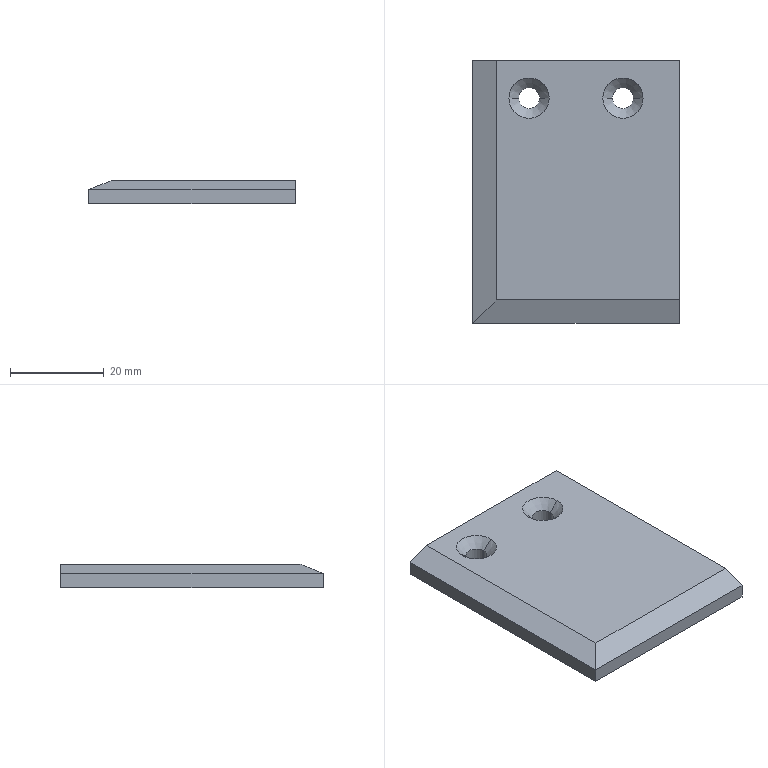Part | STEP file | PN_0027 Mount electronic clip acrylic plate | 1 solid | 16 faces | box 44 x 56 x 5 mm | volume 11600 mm3 | plane 8 | cone 4 | cylinder 4 | commonest cylinder face diameters 4.5 x4
STEP:
#1=CARTESIAN_POINT('',(0.,0.,0.));
#2=DIRECTION('',(0.,0.,1.));
#3=DIRECTION('',(1.,0.,0.));
#4=AXIS2_PLACEMENT_3D('',#1,#2,#3);
#5=CARTESIAN_POINT('',(-7.75,20.,2.95));
#6=VERTEX_POINT('',#5);
#7=CARTESIAN_POINT('',(-5.7,20.,5.));
#8=VERTEX_POINT('',#7);
#9=CARTESIAN_POINT('',(-5.7,20.,5.));
#10=DIRECTION('',(0.7071,0.,0.7071));
#11=VECTOR('',#10,1.);
#12=LINE('',#9,#11);
#13=CARTESIAN_POINT('',(-10.,20.,5.));
#14=DIRECTION('',(0.,0.,1.));
#15=DIRECTION('',(1.,0.,0.));
#16=AXIS2_PLACEMENT_3D('',#13,#14,#15);
#17=CONICAL_SURFACE('',#16,4.3,0.7854);
#18=CARTESIAN_POINT('',(6.283,0.));
#19=DIRECTION('',(0.,1.));
#20=VECTOR('',#19,1.);
#21=LINE('',#18,#20);
#22=(GEOMETRIC_REPRESENTATION_CONTEXT(2)PARAMETRIC_REPRESENTATION_CONTEXT()REPRESENTATION_CONTEXT('',''));
#23=DEFINITIONAL_REPRESENTATION('',(#21),#22);
#24=PCURVE('',#17,#23);
#25=CARTESIAN_POINT('',(-10.,20.,5.));
#26=DIRECTION('',(0.,0.,1.));
#27=DIRECTION('',(1.,0.,0.));
#28=AXIS2_PLACEMENT_3D('',#25,#26,#27);
#29=CONICAL_SURFACE('',#28,4.3,0.7854);
#30=CARTESIAN_POINT('',(0.,0.));
#31=DIRECTION('',(0.,1.));
#32=VECTOR('',#31,1.);
#33=LINE('',#30,#32);
#34=(GEOMETRIC_REPRESENTATION_CONTEXT(2)PARAMETRIC_REPRESENTATION_CONTEXT()REPRESENTATION_CONTEXT('',''));
#35=DEFINITIONAL_REPRESENTATION('',(#33),#34);
#36=PCURVE('',#29,#35);
#37=SURFACE_CURVE('',#12,(#24,#36),.PCURVE_S1.);
#38=EDGE_CURVE('',#6,#8,#37,.T.);
#39=ORIENTED_EDGE('',*,*,#38,.T.);
#40=CARTESIAN_POINT('',(-14.3,20.,5.));
#41=VERTEX_POINT('',#40);
#42=CARTESIAN_POINT('',(-10.,20.,5.));
#43=DIRECTION('',(0.,0.,1.));
#44=DIRECTION('',(1.,0.,0.));
#45=AXIS2_PLACEMENT_3D('',#42,#43,#44);
#46=CIRCLE('',#45,4.3);
#47=CARTESIAN_POINT('',(0.,0.));
#48=DIRECTION('',(1.,0.));
#49=VECTOR('',#48,1.);
#50=LINE('',#47,#49);
#51=(GEOMETRIC_REPRESENTATION_CONTEXT(2)PARAMETRIC_REPRESENTATION_CONTEXT()REPRESENTATION_CONTEXT('',''));
#52=DEFINITIONAL_REPRESENTATION('',(#50),#51);
#53=PCURVE('',#17,#52);
#54=CARTESIAN_POINT('',(0.,0.,5.));
#55=DIRECTION('',(0.,0.,-1.));
#56=DIRECTION('',(-1.,0.,0.));
#57=AXIS2_PLACEMENT_3D('',#54,#55,#56);
#58=PLANE('',#57);
#59=CARTESIAN_POINT('',(5.7,20.));
#60=CARTESIAN_POINT('',(5.7,27.448));
#61=CARTESIAN_POINT('',(12.15,23.724));
#62=CARTESIAN_POINT('',(18.6,20.));
#63=CARTESIAN_POINT('',(12.15,16.276));
#64=CARTESIAN_POINT('',(5.7,12.552));
#65=CARTESIAN_POINT('',(5.7,20.));
#66=(BOUNDED_CURVE()B_SPLINE_CURVE(2,(#59,#60,#61,#62,#63,#64,#65),.UNSPECIFIED.,.T.,.F.)B_SPLINE_CURVE_WITH_KNOTS((1,2,2,2,2,1),(-2.094,0.,2.094,4.189,6.283,8.378),.UNSPECIFIED.)CURVE()GEOMETRIC_REPRESENTATION_ITEM()RATIONAL_B_SPLINE_CURVE((1.,0.5,1.,0.5,1.,0.5,1.))REPRESENTATION_ITEM(''));
#67=(GEOMETRIC_REPRESENTATION_CONTEXT(2)PARAMETRIC_REPRESENTATION_CONTEXT()REPRESENTATION_CONTEXT('',''));
#68=DEFINITIONAL_REPRESENTATION('',(#66),#67);
#69=PCURVE('',#58,#68);
#70=SURFACE_CURVE('',#46,(#53,#69),.PCURVE_S1.);
#71=EDGE_CURVE('',#41,#8,#70,.T.);
#72=ORIENTED_EDGE('',*,*,#71,.F.);
#73=CARTESIAN_POINT('',(-12.25,20.,2.95));
#74=VERTEX_POINT('',#73);
#75=CARTESIAN_POINT('',(-14.3,20.,5.));
#76=DIRECTION('',(-0.7071,0.,0.7071));
#77=VECTOR('',#76,1.);
#78=LINE('',#75,#77);
#79=CARTESIAN_POINT('',(3.142,0.));
#80=DIRECTION('',(0.,1.));
#81=VECTOR('',#80,1.);
#82=LINE('',#79,#81);
#83=(GEOMETRIC_REPRESENTATION_CONTEXT(2)PARAMETRIC_REPRESENTATION_CONTEXT()REPRESENTATION_CONTEXT('',''));
#84=DEFINITIONAL_REPRESENTATION('',(#82),#83);
#85=PCURVE('',#17,#84);
#86=CARTESIAN_POINT('',(3.142,0.));
#87=DIRECTION('',(0.,1.));
#88=VECTOR('',#87,1.);
#89=LINE('',#86,#88);
#90=(GEOMETRIC_REPRESENTATION_CONTEXT(2)PARAMETRIC_REPRESENTATION_CONTEXT()REPRESENTATION_CONTEXT('',''));
#91=DEFINITIONAL_REPRESENTATION('',(#89),#90);
#92=PCURVE('',#29,#91);
#93=SURFACE_CURVE('',#78,(#85,#92),.PCURVE_S1.);
#94=EDGE_CURVE('',#74,#41,#93,.T.);
#95=ORIENTED_EDGE('',*,*,#94,.F.);
#96=CARTESIAN_POINT('',(-10.,20.,2.95));
#97=DIRECTION('',(0.,0.,1.));
#98=DIRECTION('',(1.,0.,0.));
#99=AXIS2_PLACEMENT_3D('',#96,#97,#98);
#100=CIRCLE('',#99,2.25);
#101=CARTESIAN_POINT('',(0.,-2.05));
#102=DIRECTION('',(1.,0.));
#103=VECTOR('',#102,1.);
#104=LINE('',#101,#103);
#105=(GEOMETRIC_REPRESENTATION_CONTEXT(2)PARAMETRIC_REPRESENTATION_CONTEXT()REPRESENTATION_CONTEXT('',''));
#106=DEFINITIONAL_REPRESENTATION('',(#104),#105);
#107=PCURVE('',#17,#106);
#108=CARTESIAN_POINT('',(-10.,20.,5.));
#109=DIRECTION('',(0.,0.,1.));
#110=DIRECTION('',(1.,0.,0.));
#111=AXIS2_PLACEMENT_3D('',#108,#109,#110);
#112=CYLINDRICAL_SURFACE('',#111,2.25);
#113=CARTESIAN_POINT('',(0.,-2.05));
#114=DIRECTION('',(1.,0.));
#115=VECTOR('',#114,1.);
#116=LINE('',#113,#115);
#117=(GEOMETRIC_REPRESENTATION_CONTEXT(2)PARAMETRIC_REPRESENTATION_CONTEXT()REPRESENTATION_CONTEXT('',''));
#118=DEFINITIONAL_REPRESENTATION('',(#116),#117);
#119=PCURVE('',#112,#118);
#120=SURFACE_CURVE('',#100,(#107,#119),.PCURVE_S1.);
#121=EDGE_CURVE('',#74,#6,#120,.T.);
#122=ORIENTED_EDGE('',*,*,#121,.T.);
#123=EDGE_LOOP('',(#39,#72,#95,#122));
#124=FACE_BOUND('',#123,.F.);
#125=ADVANCED_FACE('',(#124),#17,.F.);
#126=CARTESIAN_POINT('',(-7.75,20.,0.));
#127=VERTEX_POINT('',#126);
#128=CARTESIAN_POINT('',(-7.75,20.,5.));
#129=DIRECTION('',(0.,0.,1.));
#130=VECTOR('',#129,1.);
#131=LINE('',#128,#130);
#132=CARTESIAN_POINT('',(6.283,0.));
#133=DIRECTION('',(0.,1.));
#134=VECTOR('',#133,1.);
#135=LINE('',#132,#134);
#136=(GEOMETRIC_REPRESENTATION_CONTEXT(2)PARAMETRIC_REPRESENTATION_CONTEXT()REPRESENTATION_CONTEXT('',''));
#137=DEFINITIONAL_REPRESENTATION('',(#135),#136);
#138=PCURVE('',#112,#137);
#139=CARTESIAN_POINT('',(-10.,20.,5.));
#140=DIRECTION('',(0.,0.,1.));
#141=DIRECTION('',(1.,0.,0.));
#142=AXIS2_PLACEMENT_3D('',#139,#140,#141);
#143=CYLINDRICAL_SURFACE('',#142,2.25);
#144=CARTESIAN_POINT('',(0.,0.));
#145=DIRECTION('',(0.,1.));
#146=VECTOR('',#145,1.);
#147=LINE('',#144,#146);
#148=(GEOMETRIC_REPRESENTATION_CONTEXT(2)PARAMETRIC_REPRESENTATION_CONTEXT()REPRESENTATION_CONTEXT('',''));
#149=DEFINITIONAL_REPRESENTATION('',(#147),#148);
#150=PCURVE('',#143,#149);
#151=SURFACE_CURVE('',#131,(#138,#150),.PCURVE_S1.);
#152=EDGE_CURVE('',#127,#6,#151,.T.);
#153=ORIENTED_EDGE('',*,*,#152,.T.);
#154=ORIENTED_EDGE('',*,*,#121,.F.);
#155=CARTESIAN_POINT('',(-12.25,20.,0.));
#156=VERTEX_POINT('',#155);
#157=CARTESIAN_POINT('',(-12.25,20.,5.));
#158=DIRECTION('',(0.,0.,1.));
#159=VECTOR('',#158,1.);
#160=LINE('',#157,#159);
#161=CARTESIAN_POINT('',(3.142,0.));
#162=DIRECTION('',(0.,1.));
#163=VECTOR('',#162,1.);
#164=LINE('',#161,#163);
#165=(GEOMETRIC_REPRESENTATION_CONTEXT(2)PARAMETRIC_REPRESENTATION_CONTEXT()REPRESENTATION_CONTEXT('',''));
#166=DEFINITIONAL_REPRESENTATION('',(#164),#165);
#167=PCURVE('',#112,#166);
#168=CARTESIAN_POINT('',(3.142,0.));
#169=DIRECTION('',(0.,1.));
#170=VECTOR('',#169,1.);
#171=LINE('',#168,#170);
#172=(GEOMETRIC_REPRESENTATION_CONTEXT(2)PARAMETRIC_REPRESENTATION_CONTEXT()REPRESENTATION_CONTEXT('',''));
#173=DEFINITIONAL_REPRESENTATION('',(#171),#172);
#174=PCURVE('',#143,#173);
#175=SURFACE_CURVE('',#160,(#167,#174),.PCURVE_S1.);
#176=EDGE_CURVE('',#156,#74,#175,.T.);
#177=ORIENTED_EDGE('',*,*,#176,.F.);
#178=CARTESIAN_POINT('',(-10.,20.,0.));
#179=DIRECTION('',(0.,0.,1.));
#180=DIRECTION('',(1.,0.,0.));
#181=AXIS2_PLACEMENT_3D('',#178,#179,#180);
#182=CIRCLE('',#181,2.25);
#183=CARTESIAN_POINT('',(0.,-5.));
#184=DIRECTION('',(1.,0.));
#185=VECTOR('',#184,1.);
#186=LINE('',#183,#185);
#187=(GEOMETRIC_REPRESENTATION_CONTEXT(2)PARAMETRIC_REPRESENTATION_CONTEXT()REPRESENTATION_CONTEXT('',''));
#188=DEFINITIONAL_REPRESENTATION('',(#186),#187);
#189=PCURVE('',#112,#188);
#190=CARTESIAN_POINT('',(0.,0.,0.));
#191=DIRECTION('',(0.,0.,-1.));
#192=DIRECTION('',(-1.,0.,0.));
#193=AXIS2_PLACEMENT_3D('',#190,#191,#192);
#194=PLANE('',#193);
#195=CARTESIAN_POINT('',(7.75,20.));
#196=CARTESIAN_POINT('',(7.75,23.897));
#197=CARTESIAN_POINT('',(11.125,21.949));
#198=CARTESIAN_POINT('',(14.5,20.));
#199=CARTESIAN_POINT('',(11.125,18.051));
#200=CARTESIAN_POINT('',(7.75,16.103));
#201=CARTESIAN_POINT('',(7.75,20.));
#202=(BOUNDED_CURVE()B_SPLINE_CURVE(2,(#195,#196,#197,#198,#199,#200,#201),.UNSPECIFIED.,.T.,.F.)B_SPLINE_CURVE_WITH_KNOTS((1,2,2,2,2,1),(-2.094,0.,2.094,4.189,6.283,8.378),.UNSPECIFIED.)CURVE()GEOMETRIC_REPRESENTATION_ITEM()RATIONAL_B_SPLINE_CURVE((1.,0.5,1.,0.5,1.,0.5,1.))REPRESENTATION_ITEM(''));
#203=(GEOMETRIC_REPRESENTATION_CONTEXT(2)PARAMETRIC_REPRESENTATION_CONTEXT()REPRESENTATION_CONTEXT('',''));
#204=DEFINITIONAL_REPRESENTATION('',(#202),#203);
#205=PCURVE('',#194,#204);
#206=SURFACE_CURVE('',#182,(#189,#205),.PCURVE_S1.);
#207=EDGE_CURVE('',#156,#127,#206,.T.);
#208=ORIENTED_EDGE('',*,*,#207,.T.);
#209=EDGE_LOOP('',(#153,#154,#177,#208));
#210=FACE_BOUND('',#209,.F.);
#211=ADVANCED_FACE('',(#210),#112,.F.);
#212=CARTESIAN_POINT('',(12.25,20.,2.95));
#213=VERTEX_POINT('',#212);
#214=CARTESIAN_POINT('',(14.3,20.,5.));
#215=VERTEX_POINT('',#214);
#216=CARTESIAN_POINT('',(14.3,20.,5.));
#217=DIRECTION('',(0.7071,0.,0.7071));
#218=VECTOR('',#217,1.);
#219=LINE('',#216,#218);
#220=CARTESIAN_POINT('',(10.,20.,5.));
#221=DIRECTION('',(0.,0.,1.));
#222=DIRECTION('',(1.,0.,0.));
#223=AXIS2_PLACEMENT_3D('',#220,#221,#222);
#224=CONICAL_SURFACE('',#223,4.3,0.7854);
#225=CARTESIAN_POINT('',(6.283,0.));
#226=DIRECTION('',(0.,1.));
#227=VECTOR('',#226,1.);
#228=LINE('',#225,#227);
#229=(GEOMETRIC_REPRESENTATION_CONTEXT(2)PARAMETRIC_REPRESENTATION_CONTEXT()REPRESENTATION_CONTEXT('',''));
#230=DEFINITIONAL_REPRESENTATION('',(#228),#229);
#231=PCURVE('',#224,#230);
#232=CARTESIAN_POINT('',(10.,20.,5.));
#233=DIRECTION('',(0.,0.,1.));
#234=DIRECTION('',(1.,0.,0.));
#235=AXIS2_PLACEMENT_3D('',#232,#233,#234);
#236=CONICAL_SURFACE('',#235,4.3,0.7854);
#237=CARTESIAN_POINT('',(0.,0.));
#238=DIRECTION('',(0.,1.));
#239=VECTOR('',#238,1.);
#240=LINE('',#237,#239);
#241=(GEOMETRIC_REPRESENTATION_CONTEXT(2)PARAMETRIC_REPRESENTATION_CONTEXT()REPRESENTATION_CONTEXT('',''));
#242=DEFINITIONAL_REPRESENTATION('',(#240),#241);
#243=PCURVE('',#236,#242);
#244=SURFACE_CURVE('',#219,(#231,#243),.PCURVE_S1.);
#245=EDGE_CURVE('',#213,#215,#244,.T.);
#246=ORIENTED_EDGE('',*,*,#245,.T.);
#247=CARTESIAN_POINT('',(5.7,20.,5.));
#248=VERTEX_POINT('',#247);
#249=CARTESIAN_POINT('',(10.,20.,5.));
#250=DIRECTION('',(0.,0.,1.));
#251=DIRECTION('',(1.,0.,0.));
#252=AXIS2_PLACEMENT_3D('',#249,#250,#251);
#253=CIRCLE('',#252,4.3);
#254=CARTESIAN_POINT('',(0.,0.));
#255=DIRECTION('',(1.,0.));
#256=VECTOR('',#255,1.);
#257=LINE('',#254,#256);
#258=(GEOMETRIC_REPRESENTATION_CONTEXT(2)PARAMETRIC_REPRESENTATION_CONTEXT()REPRESENTATION_CONTEXT('',''));
#259=DEFINITIONAL_REPRESENTATION('',(#257),#258);
#260=PCURVE('',#224,#259);
#261=CARTESIAN_POINT('',(-14.3,20.));
#262=CARTESIAN_POINT('',(-14.3,27.448));
#263=CARTESIAN_POINT('',(-7.85,23.724));
#264=CARTESIAN_POINT('',(-1.4,20.));
#265=CARTESIAN_POINT('',(-7.85,16.276));
#266=CARTESIAN_POINT('',(-14.3,12.552));
#267=CARTESIAN_POINT('',(-14.3,20.));
#268=(BOUNDED_CURVE()B_SPLINE_CURVE(2,(#261,#262,#263,#264,#265,#266,#267),.UNSPECIFIED.,.T.,.F.)B_SPLINE_CURVE_WITH_KNOTS((1,2,2,2,2,1),(-2.094,0.,2.094,4.189,6.283,8.378),.UNSPECIFIED.)CURVE()GEOMETRIC_REPRESENTATION_ITEM()RATIONAL_B_SPLINE_CURVE((1.,0.5,1.,0.5,1.,0.5,1.))REPRESENTATION_ITEM(''));
#269=(GEOMETRIC_REPRESENTATION_CONTEXT(2)PARAMETRIC_REPRESENTATION_CONTEXT()REPRESENTATION_CONTEXT('',''));
#270=DEFINITIONAL_REPRESENTATION('',(#268),#269);
#271=PCURVE('',#58,#270);
#272=SURFACE_CURVE('',#253,(#260,#271),.PCURVE_S1.);
#273=EDGE_CURVE('',#248,#215,#272,.T.);
#274=ORIENTED_EDGE('',*,*,#273,.F.);
#275=CARTESIAN_POINT('',(7.75,20.,2.95));
#276=VERTEX_POINT('',#275);
#277=CARTESIAN_POINT('',(5.7,20.,5.));
#278=DIRECTION('',(-0.7071,0.,0.7071));
#279=VECTOR('',#278,1.);
#280=LINE('',#277,#279);
#281=CARTESIAN_POINT('',(3.142,0.));
#282=DIRECTION('',(0.,1.));
#283=VECTOR('',#282,1.);
#284=LINE('',#281,#283);
#285=(GEOMETRIC_REPRESENTATION_CONTEXT(2)PARAMETRIC_REPRESENTATION_CONTEXT()REPRESENTATION_CONTEXT('',''));
#286=DEFINITIONAL_REPRESENTATION('',(#284),#285);
#287=PCURVE('',#224,#286);
#288=CARTESIAN_POINT('',(3.142,0.));
#289=DIRECTION('',(0.,1.));
#290=VECTOR('',#289,1.);
#291=LINE('',#288,#290);
#292=(GEOMETRIC_REPRESENTATION_CONTEXT(2)PARAMETRIC_REPRESENTATION_CONTEXT()REPRESENTATION_CONTEXT('',''));
#293=DEFINITIONAL_REPRESENTATION('',(#291),#292);
#294=PCURVE('',#236,#293);
#295=SURFACE_CURVE('',#280,(#287,#294),.PCURVE_S1.);
#296=EDGE_CURVE('',#276,#248,#295,.T.);
#297=ORIENTED_EDGE('',*,*,#296,.F.);
#298=CARTESIAN_POINT('',(10.,20.,2.95));
#299=DIRECTION('',(0.,0.,1.));
#300=DIRECTION('',(1.,0.,0.));
#301=AXIS2_PLACEMENT_3D('',#298,#299,#300);
#302=CIRCLE('',#301,2.25);
#303=CARTESIAN_POINT('',(0.,-2.05));
#304=DIRECTION('',(1.,0.));
#305=VECTOR('',#304,1.);
#306=LINE('',#303,#305);
#307=(GEOMETRIC_REPRESENTATION_CONTEXT(2)PARAMETRIC_REPRESENTATION_CONTEXT()REPRESENTATION_CONTEXT('',''));
#308=DEFINITIONAL_REPRESENTATION('',(#306),#307);
#309=PCURVE('',#224,#308);
#310=CARTESIAN_POINT('',(10.,20.,5.));
#311=DIRECTION('',(0.,0.,1.));
#312=DIRECTION('',(1.,0.,0.));
#313=AXIS2_PLACEMENT_3D('',#310,#311,#312);
#314=CYLINDRICAL_SURFACE('',#313,2.25);
#315=CARTESIAN_POINT('',(0.,-2.05));
#316=DIRECTION('',(1.,0.));
#317=VECTOR('',#316,1.);
#318=LINE('',#315,#317);
#319=(GEOMETRIC_REPRESENTATION_CONTEXT(2)PARAMETRIC_REPRESENTATION_CONTEXT()REPRESENTATION_CONTEXT('',''));
#320=DEFINITIONAL_REPRESENTATION('',(#318),#319);
#321=PCURVE('',#314,#320);
#322=SURFACE_CURVE('',#302,(#309,#321),.PCURVE_S1.);
#323=EDGE_CURVE('',#276,#213,#322,.T.);
#324=ORIENTED_EDGE('',*,*,#323,.T.);
#325=EDGE_LOOP('',(#246,#274,#297,#324));
#326=FACE_BOUND('',#325,.F.);
#327=ADVANCED_FACE('',(#326),#224,.F.);
#328=CARTESIAN_POINT('',(12.25,20.,0.));
#329=VERTEX_POINT('',#328);
#330=CARTESIAN_POINT('',(12.25,20.,5.));
#331=DIRECTION('',(0.,0.,1.));
#332=VECTOR('',#331,1.);
#333=LINE('',#330,#332);
#334=CARTESIAN_POINT('',(6.283,0.));
#335=DIRECTION('',(0.,1.));
#336=VECTOR('',#335,1.);
#337=LINE('',#334,#336);
#338=(GEOMETRIC_REPRESENTATION_CONTEXT(2)PARAMETRIC_REPRESENTATION_CONTEXT()REPRESENTATION_CONTEXT('',''));
#339=DEFINITIONAL_REPRESENTATION('',(#337),#338);
#340=PCURVE('',#314,#339);
#341=CARTESIAN_POINT('',(10.,20.,5.));
#342=DIRECTION('',(0.,0.,1.));
#343=DIRECTION('',(1.,0.,0.));
#344=AXIS2_PLACEMENT_3D('',#341,#342,#343);
#345=CYLINDRICAL_SURFACE('',#344,2.25);
#346=CARTESIAN_POINT('',(0.,0.));
#347=DIRECTION('',(0.,1.));
#348=VECTOR('',#347,1.);
#349=LINE('',#346,#348);
#350=(GEOMETRIC_REPRESENTATION_CONTEXT(2)PARAMETRIC_REPRESENTATION_CONTEXT()REPRESENTATION_CONTEXT('',''));
#351=DEFINITIONAL_REPRESENTATION('',(#349),#350);
#352=PCURVE('',#345,#351);
#353=SURFACE_CURVE('',#333,(#340,#352),.PCURVE_S1.);
#354=EDGE_CURVE('',#329,#213,#353,.T.);
#355=ORIENTED_EDGE('',*,*,#354,.T.);
#356=ORIENTED_EDGE('',*,*,#323,.F.);
#357=CARTESIAN_POINT('',(7.75,20.,0.));
#358=VERTEX_POINT('',#357);
#359=CARTESIAN_POINT('',(7.75,20.,5.));
#360=DIRECTION('',(0.,0.,1.));
#361=VECTOR('',#360,1.);
#362=LINE('',#359,#361);
#363=CARTESIAN_POINT('',(3.142,0.));
#364=DIRECTION('',(0.,1.));
#365=VECTOR('',#364,1.);
#366=LINE('',#363,#365);
#367=(GEOMETRIC_REPRESENTATION_CONTEXT(2)PARAMETRIC_REPRESENTATION_CONTEXT()REPRESENTATION_CONTEXT('',''));
#368=DEFINITIONAL_REPRESENTATION('',(#366),#367);
#369=PCURVE('',#314,#368);
#370=CARTESIAN_POINT('',(3.142,0.));
#371=DIRECTION('',(0.,1.));
#372=VECTOR('',#371,1.);
#373=LINE('',#370,#372);
#374=(GEOMETRIC_REPRESENTATION_CONTEXT(2)PARAMETRIC_REPRESENTATION_CONTEXT()REPRESENTATION_CONTEXT('',''));
#375=DEFINITIONAL_REPRESENTATION('',(#373),#374);
#376=PCURVE('',#345,#375);
#377=SURFACE_CURVE('',#362,(#369,#376),.PCURVE_S1.);
#378=EDGE_CURVE('',#358,#276,#377,.T.);
#379=ORIENTED_EDGE('',*,*,#378,.F.);
#380=CARTESIAN_POINT('',(10.,20.,0.));
#381=DIRECTION('',(0.,0.,1.));
#382=DIRECTION('',(1.,0.,0.));
#383=AXIS2_PLACEMENT_3D('',#380,#381,#382);
#384=CIRCLE('',#383,2.25);
#385=CARTESIAN_POINT('',(0.,-5.));
#386=DIRECTION('',(1.,0.));
#387=VECTOR('',#386,1.);
#388=LINE('',#385,#387);
#389=(GEOMETRIC_REPRESENTATION_CONTEXT(2)PARAMETRIC_REPRESENTATION_CONTEXT()REPRESENTATION_CONTEXT('',''));
#390=DEFINITIONAL_REPRESENTATION('',(#388),#389);
#391=PCURVE('',#314,#390);
#392=CARTESIAN_POINT('',(-12.25,20.));
#393=CARTESIAN_POINT('',(-12.25,23.897));
#394=CARTESIAN_POINT('',(-8.875,21.949));
#395=CARTESIAN_POINT('',(-5.5,20.));
#396=CARTESIAN_POINT('',(-8.875,18.051));
#397=CARTESIAN_POINT('',(-12.25,16.103));
#398=CARTESIAN_POINT('',(-12.25,20.));
#399=(BOUNDED_CURVE()B_SPLINE_CURVE(2,(#392,#393,#394,#395,#396,#397,#398),.UNSPECIFIED.,.T.,.F.)B_SPLINE_CURVE_WITH_KNOTS((1,2,2,2,2,1),(-2.094,0.,2.094,4.189,6.283,8.378),.UNSPECIFIED.)CURVE()GEOMETRIC_REPRESENTATION_ITEM()RATIONAL_B_SPLINE_CURVE((1.,0.5,1.,0.5,1.,0.5,1.))REPRESENTATION_ITEM(''));
#400=(GEOMETRIC_REPRESENTATION_CONTEXT(2)PARAMETRIC_REPRESENTATION_CONTEXT()REPRESENTATION_CONTEXT('',''));
#401=DEFINITIONAL_REPRESENTATION('',(#399),#400);
#402=PCURVE('',#194,#401);
#403=SURFACE_CURVE('',#384,(#391,#402),.PCURVE_S1.);
#404=EDGE_CURVE('',#358,#329,#403,.T.);
#405=ORIENTED_EDGE('',*,*,#404,.T.);
#406=EDGE_LOOP('',(#355,#356,#379,#405));
#407=FACE_BOUND('',#406,.F.);
#408=ADVANCED_FACE('',(#407),#314,.F.);
#409=CARTESIAN_POINT('',(22.,-23.,5.));
#410=VERTEX_POINT('',#409);
#411=CARTESIAN_POINT('',(22.,28.,5.));
#412=VERTEX_POINT('',#411);
#413=CARTESIAN_POINT('',(22.,-28.,5.));
#414=DIRECTION('',(0.,1.,0.));
#415=VECTOR('',#414,1.);
#416=LINE('',#413,#415);
#417=CARTESIAN_POINT('',(22.,-28.,5.));
#418=DIRECTION('',(-1.,0.,0.));
#419=DIRECTION('',(0.,0.,1.));
#420=AXIS2_PLACEMENT_3D('',#417,#418,#419);
#421=PLANE('',#420);
#422=CARTESIAN_POINT('',(0.,0.));
#423=DIRECTION('',(0.,1.));
#424=VECTOR('',#423,1.);
#425=LINE('',#422,#424);
#426=(GEOMETRIC_REPRESENTATION_CONTEXT(2)PARAMETRIC_REPRESENTATION_CONTEXT()REPRESENTATION_CONTEXT('',''));
#427=DEFINITIONAL_REPRESENTATION('',(#425),#426);
#428=PCURVE('',#421,#427);
#429=CARTESIAN_POINT('',(-22.,-28.));
#430=DIRECTION('',(0.,1.));
#431=VECTOR('',#430,1.);
#432=LINE('',#429,#431);
#433=(GEOMETRIC_REPRESENTATION_CONTEXT(2)PARAMETRIC_REPRESENTATION_CONTEXT()REPRESENTATION_CONTEXT('',''));
#434=DEFINITIONAL_REPRESENTATION('',(#432),#433);
#435=PCURVE('',#58,#434);
#436=SURFACE_CURVE('',#416,(#428,#435),.PCURVE_S1.);
#437=EDGE_CURVE('',#410,#412,#436,.T.);
#438=ORIENTED_EDGE('',*,*,#437,.F.);
#439=CARTESIAN_POINT('',(22.,-28.,3.));
#440=VERTEX_POINT('',#439);
#441=CARTESIAN_POINT('',(22.,-23.,5.));
#442=DIRECTION('',(0.,-0.9285,-0.3714));
#443=VECTOR('',#442,1.);
#444=LINE('',#441,#443);
#445=CARTESIAN_POINT('',(0.,5.));
#446=DIRECTION('',(-0.3714,-0.9285));
#447=VECTOR('',#446,1.);
#448=LINE('',#445,#447);
#449=(GEOMETRIC_REPRESENTATION_CONTEXT(2)PARAMETRIC_REPRESENTATION_CONTEXT()REPRESENTATION_CONTEXT('',''));
#450=DEFINITIONAL_REPRESENTATION('',(#448),#449);
#451=PCURVE('',#421,#450);
#452=CARTESIAN_POINT('',(0.,-23.,5.));
#453=DIRECTION('',(0.,0.3714,-0.9285));
#454=DIRECTION('',(1.,0.,0.));
#455=AXIS2_PLACEMENT_3D('',#452,#453,#454);
#456=PLANE('',#455);
#457=CARTESIAN_POINT('',(22.,0.));
#458=DIRECTION('',(0.,1.));
#459=VECTOR('',#458,1.);
#460=LINE('',#457,#459);
#461=(GEOMETRIC_REPRESENTATION_CONTEXT(2)PARAMETRIC_REPRESENTATION_CONTEXT()REPRESENTATION_CONTEXT('',''));
#462=DEFINITIONAL_REPRESENTATION('',(#460),#461);
#463=PCURVE('',#456,#462);
#464=SURFACE_CURVE('',#444,(#451,#463),.PCURVE_S1.);
#465=EDGE_CURVE('',#410,#440,#464,.T.);
#466=ORIENTED_EDGE('',*,*,#465,.T.);
#467=CARTESIAN_POINT('',(22.,-28.,0.));
#468=VERTEX_POINT('',#467);
#469=CARTESIAN_POINT('',(22.,-28.,5.));
#470=DIRECTION('',(0.,0.,-1.));
#471=VECTOR('',#470,1.);
#472=LINE('',#469,#471);
#473=CARTESIAN_POINT('',(0.,0.));
#474=DIRECTION('',(-1.,0.));
#475=VECTOR('',#474,1.);
#476=LINE('',#473,#475);
#477=(GEOMETRIC_REPRESENTATION_CONTEXT(2)PARAMETRIC_REPRESENTATION_CONTEXT()REPRESENTATION_CONTEXT('',''));
#478=DEFINITIONAL_REPRESENTATION('',(#476),#477);
#479=PCURVE('',#421,#478);
#480=CARTESIAN_POINT('',(-22.,-28.,5.));
#481=DIRECTION('',(0.,1.,0.));
#482=DIRECTION('',(0.,0.,1.));
#483=AXIS2_PLACEMENT_3D('',#480,#481,#482);
#484=PLANE('',#483);
#485=CARTESIAN_POINT('',(0.,44.));
#486=DIRECTION('',(-1.,0.));
#487=VECTOR('',#486,1.);
#488=LINE('',#485,#487);
#489=(GEOMETRIC_REPRESENTATION_CONTEXT(2)PARAMETRIC_REPRESENTATION_CONTEXT()REPRESENTATION_CONTEXT('',''));
#490=DEFINITIONAL_REPRESENTATION('',(#488),#489);
#491=PCURVE('',#484,#490);
#492=SURFACE_CURVE('',#472,(#479,#491),.PCURVE_S1.);
#493=EDGE_CURVE('',#440,#468,#492,.T.);
#494=ORIENTED_EDGE('',*,*,#493,.T.);
#495=CARTESIAN_POINT('',(22.,28.,0.));
#496=VERTEX_POINT('',#495);
#497=CARTESIAN_POINT('',(22.,-28.,0.));
#498=DIRECTION('',(0.,1.,0.));
#499=VECTOR('',#498,1.);
#500=LINE('',#497,#499);
#501=CARTESIAN_POINT('',(-5.,0.));
#502=DIRECTION('',(0.,1.));
#503=VECTOR('',#502,1.);
#504=LINE('',#501,#503);
#505=(GEOMETRIC_REPRESENTATION_CONTEXT(2)PARAMETRIC_REPRESENTATION_CONTEXT()REPRESENTATION_CONTEXT('',''));
#506=DEFINITIONAL_REPRESENTATION('',(#504),#505);
#507=PCURVE('',#421,#506);
#508=CARTESIAN_POINT('',(-22.,-28.));
#509=DIRECTION('',(0.,1.));
#510=VECTOR('',#509,1.);
#511=LINE('',#508,#510);
#512=(GEOMETRIC_REPRESENTATION_CONTEXT(2)PARAMETRIC_REPRESENTATION_CONTEXT()REPRESENTATION_CONTEXT('',''));
#513=DEFINITIONAL_REPRESENTATION('',(#511),#512);
#514=PCURVE('',#194,#513);
#515=SURFACE_CURVE('',#500,(#507,#514),.PCURVE_S1.);
#516=EDGE_CURVE('',#468,#496,#515,.T.);
#517=ORIENTED_EDGE('',*,*,#516,.T.);
#518=CARTESIAN_POINT('',(22.,28.,5.));
#519=DIRECTION('',(0.,0.,-1.));
#520=VECTOR('',#519,1.);
#521=LINE('',#518,#520);
#522=CARTESIAN_POINT('',(0.,56.));
#523=DIRECTION('',(-1.,0.));
#524=VECTOR('',#523,1.);
#525=LINE('',#522,#524);
#526=(GEOMETRIC_REPRESENTATION_CONTEXT(2)PARAMETRIC_REPRESENTATION_CONTEXT()REPRESENTATION_CONTEXT('',''));
#527=DEFINITIONAL_REPRESENTATION('',(#525),#526);
#528=PCURVE('',#421,#527);
#529=CARTESIAN_POINT('',(-22.,28.,5.));
#530=DIRECTION('',(0.,-1.,0.));
#531=DIRECTION('',(0.,0.,-1.));
#532=AXIS2_PLACEMENT_3D('',#529,#530,#531);
#533=PLANE('',#532);
#534=CARTESIAN_POINT('',(0.,44.));
#535=DIRECTION('',(1.,0.));
#536=VECTOR('',#535,1.);
#537=LINE('',#534,#536);
#538=(GEOMETRIC_REPRESENTATION_CONTEXT(2)PARAMETRIC_REPRESENTATION_CONTEXT()REPRESENTATION_CONTEXT('',''));
#539=DEFINITIONAL_REPRESENTATION('',(#537),#538);
#540=PCURVE('',#533,#539);
#541=SURFACE_CURVE('',#521,(#528,#540),.PCURVE_S1.);
#542=EDGE_CURVE('',#412,#496,#541,.T.);
#543=ORIENTED_EDGE('',*,*,#542,.F.);
#544=EDGE_LOOP('',(#438,#466,#494,#517,#543));
#545=FACE_BOUND('',#544,.T.);
#546=ADVANCED_FACE('',(#545),#421,.F.);
#547=CARTESIAN_POINT('',(-22.,28.,3.));
#548=VERTEX_POINT('',#547);
#549=CARTESIAN_POINT('',(-22.,28.,0.));
#550=VERTEX_POINT('',#549);
#551=CARTESIAN_POINT('',(-22.,28.,5.));
#552=DIRECTION('',(0.,0.,-1.));
#553=VECTOR('',#552,1.);
#554=LINE('',#551,#553);
#555=CARTESIAN_POINT('',(0.,0.));
#556=DIRECTION('',(1.,0.));
#557=VECTOR('',#556,1.);
#558=LINE('',#555,#557);
#559=(GEOMETRIC_REPRESENTATION_CONTEXT(2)PARAMETRIC_REPRESENTATION_CONTEXT()REPRESENTATION_CONTEXT('',''));
#560=DEFINITIONAL_REPRESENTATION('',(#558),#559);
#561=PCURVE('',#533,#560);
#562=CARTESIAN_POINT('',(-22.,-28.,5.));
#563=DIRECTION('',(1.,0.,0.));
#564=DIRECTION('',(0.,0.,-1.));
#565=AXIS2_PLACEMENT_3D('',#562,#563,#564);
#566=PLANE('',#565);
#567=CARTESIAN_POINT('',(0.,56.));
#568=DIRECTION('',(1.,0.));
#569=VECTOR('',#568,1.);
#570=LINE('',#567,#569);
#571=(GEOMETRIC_REPRESENTATION_CONTEXT(2)PARAMETRIC_REPRESENTATION_CONTEXT()REPRESENTATION_CONTEXT('',''));
#572=DEFINITIONAL_REPRESENTATION('',(#570),#571);
#573=PCURVE('',#566,#572);
#574=SURFACE_CURVE('',#554,(#561,#573),.PCURVE_S1.);
#575=EDGE_CURVE('',#548,#550,#574,.T.);
#576=ORIENTED_EDGE('',*,*,#575,.F.);
#577=CARTESIAN_POINT('',(-17.,28.,5.));
#578=VERTEX_POINT('',#577);
#579=CARTESIAN_POINT('',(-17.,28.,5.));
#580=DIRECTION('',(0.9285,0.,0.3714));
#581=VECTOR('',#580,1.);
#582=LINE('',#579,#581);
#583=CARTESIAN_POINT('',(0.,5.));
#584=DIRECTION('',(-0.3714,0.9285));
#585=VECTOR('',#584,1.);
#586=LINE('',#583,#585);
#587=(GEOMETRIC_REPRESENTATION_CONTEXT(2)PARAMETRIC_REPRESENTATION_CONTEXT()REPRESENTATION_CONTEXT('',''));
#588=DEFINITIONAL_REPRESENTATION('',(#586),#587);
#589=PCURVE('',#533,#588);
#590=CARTESIAN_POINT('',(-17.,0.,5.));
#591=DIRECTION('',(0.3714,0.,-0.9285));
#592=DIRECTION('',(0.,-1.,0.));
#593=AXIS2_PLACEMENT_3D('',#590,#591,#592);
#594=PLANE('',#593);
#595=CARTESIAN_POINT('',(-28.,0.));
#596=DIRECTION('',(0.,-1.));
#597=VECTOR('',#596,1.);
#598=LINE('',#595,#597);
#599=(GEOMETRIC_REPRESENTATION_CONTEXT(2)PARAMETRIC_REPRESENTATION_CONTEXT()REPRESENTATION_CONTEXT('',''));
#600=DEFINITIONAL_REPRESENTATION('',(#598),#599);
#601=PCURVE('',#594,#600);
#602=SURFACE_CURVE('',#582,(#589,#601),.PCURVE_S1.);
#603=EDGE_CURVE('',#548,#578,#602,.T.);
#604=ORIENTED_EDGE('',*,*,#603,.T.);
#605=CARTESIAN_POINT('',(-22.,28.,5.));
#606=DIRECTION('',(-1.,0.,0.));
#607=VECTOR('',#606,1.);
#608=LINE('',#605,#607);
#609=CARTESIAN_POINT('',(0.,0.));
#610=DIRECTION('',(0.,-1.));
#611=VECTOR('',#610,1.);
#612=LINE('',#609,#611);
#613=(GEOMETRIC_REPRESENTATION_CONTEXT(2)PARAMETRIC_REPRESENTATION_CONTEXT()REPRESENTATION_CONTEXT('',''));
#614=DEFINITIONAL_REPRESENTATION('',(#612),#613);
#615=PCURVE('',#533,#614);
#616=CARTESIAN_POINT('',(22.,28.));
#617=DIRECTION('',(1.,0.));
#618=VECTOR('',#617,1.);
#619=LINE('',#616,#618);
#620=(GEOMETRIC_REPRESENTATION_CONTEXT(2)PARAMETRIC_REPRESENTATION_CONTEXT()REPRESENTATION_CONTEXT('',''));
#621=DEFINITIONAL_REPRESENTATION('',(#619),#620);
#622=PCURVE('',#58,#621);
#623=SURFACE_CURVE('',#608,(#615,#622),.PCURVE_S1.);
#624=EDGE_CURVE('',#412,#578,#623,.T.);
#625=ORIENTED_EDGE('',*,*,#624,.F.);
#626=ORIENTED_EDGE('',*,*,#542,.T.);
#627=CARTESIAN_POINT('',(-22.,28.,0.));
#628=DIRECTION('',(-1.,0.,0.));
#629=VECTOR('',#628,1.);
#630=LINE('',#627,#629);
#631=CARTESIAN_POINT('',(5.,0.));
#632=DIRECTION('',(0.,-1.));
#633=VECTOR('',#632,1.);
#634=LINE('',#631,#633);
#635=(GEOMETRIC_REPRESENTATION_CONTEXT(2)PARAMETRIC_REPRESENTATION_CONTEXT()REPRESENTATION_CONTEXT('',''));
#636=DEFINITIONAL_REPRESENTATION('',(#634),#635);
#637=PCURVE('',#533,#636);
#638=CARTESIAN_POINT('',(22.,28.));
#639=DIRECTION('',(1.,0.));
#640=VECTOR('',#639,1.);
#641=LINE('',#638,#640);
#642=(GEOMETRIC_REPRESENTATION_CONTEXT(2)PARAMETRIC_REPRESENTATION_CONTEXT()REPRESENTATION_CONTEXT('',''));
#643=DEFINITIONAL_REPRESENTATION('',(#641),#642);
#644=PCURVE('',#194,#643);
#645=SURFACE_CURVE('',#630,(#637,#644),.PCURVE_S1.);
#646=EDGE_CURVE('',#496,#550,#645,.T.);
#647=ORIENTED_EDGE('',*,*,#646,.T.);
#648=EDGE_LOOP('',(#576,#604,#625,#626,#647));
#649=FACE_BOUND('',#648,.T.);
#650=ADVANCED_FACE('',(#649),#533,.F.);
#651=CARTESIAN_POINT('',(-22.,-28.,3.));
#652=VERTEX_POINT('',#651);
#653=CARTESIAN_POINT('',(-22.,-28.,0.));
#654=VERTEX_POINT('',#653);
#655=CARTESIAN_POINT('',(-22.,-28.,5.));
#656=DIRECTION('',(0.,0.,-1.));
#657=VECTOR('',#656,1.);
#658=LINE('',#655,#657);
#659=CARTESIAN_POINT('',(0.,0.));
#660=DIRECTION('',(1.,0.));
#661=VECTOR('',#660,1.);
#662=LINE('',#659,#661);
#663=(GEOMETRIC_REPRESENTATION_CONTEXT(2)PARAMETRIC_REPRESENTATION_CONTEXT()REPRESENTATION_CONTEXT('',''));
#664=DEFINITIONAL_REPRESENTATION('',(#662),#663);
#665=PCURVE('',#566,#664);
#666=CARTESIAN_POINT('',(0.,0.));
#667=DIRECTION('',(-1.,0.));
#668=VECTOR('',#667,1.);
#669=LINE('',#666,#668);
#670=(GEOMETRIC_REPRESENTATION_CONTEXT(2)PARAMETRIC_REPRESENTATION_CONTEXT()REPRESENTATION_CONTEXT('',''));
#671=DEFINITIONAL_REPRESENTATION('',(#669),#670);
#672=PCURVE('',#484,#671);
#673=SURFACE_CURVE('',#658,(#665,#672),.PCURVE_S1.);
#674=EDGE_CURVE('',#652,#654,#673,.T.);
#675=ORIENTED_EDGE('',*,*,#674,.F.);
#676=CARTESIAN_POINT('',(-22.,-28.,3.));
#677=DIRECTION('',(0.,1.,0.));
#678=VECTOR('',#677,1.);
#679=LINE('',#676,#678);
#680=CARTESIAN_POINT('',(2.,0.));
#681=DIRECTION('',(0.,1.));
#682=VECTOR('',#681,1.);
#683=LINE('',#680,#682);
#684=(GEOMETRIC_REPRESENTATION_CONTEXT(2)PARAMETRIC_REPRESENTATION_CONTEXT()REPRESENTATION_CONTEXT('',''));
#685=DEFINITIONAL_REPRESENTATION('',(#683),#684);
#686=PCURVE('',#566,#685);
#687=CARTESIAN_POINT('',(28.,5.385));
#688=DIRECTION('',(-1.,0.));
#689=VECTOR('',#688,1.);
#690=LINE('',#687,#689);
#691=(GEOMETRIC_REPRESENTATION_CONTEXT(2)PARAMETRIC_REPRESENTATION_CONTEXT()REPRESENTATION_CONTEXT('',''));
#692=DEFINITIONAL_REPRESENTATION('',(#690),#691);
#693=PCURVE('',#594,#692);
#694=SURFACE_CURVE('',#679,(#686,#693),.PCURVE_S1.);
#695=EDGE_CURVE('',#652,#548,#694,.T.);
#696=ORIENTED_EDGE('',*,*,#695,.T.);
#697=ORIENTED_EDGE('',*,*,#575,.T.);
#698=CARTESIAN_POINT('',(-22.,-28.,0.));
#699=DIRECTION('',(0.,-1.,0.));
#700=VECTOR('',#699,1.);
#701=LINE('',#698,#700);
#702=CARTESIAN_POINT('',(5.,0.));
#703=DIRECTION('',(0.,-1.));
#704=VECTOR('',#703,1.);
#705=LINE('',#702,#704);
#706=(GEOMETRIC_REPRESENTATION_CONTEXT(2)PARAMETRIC_REPRESENTATION_CONTEXT()REPRESENTATION_CONTEXT('',''));
#707=DEFINITIONAL_REPRESENTATION('',(#705),#706);
#708=PCURVE('',#566,#707);
#709=CARTESIAN_POINT('',(22.,-28.));
#710=DIRECTION('',(0.,-1.));
#711=VECTOR('',#710,1.);
#712=LINE('',#709,#711);
#713=(GEOMETRIC_REPRESENTATION_CONTEXT(2)PARAMETRIC_REPRESENTATION_CONTEXT()REPRESENTATION_CONTEXT('',''));
#714=DEFINITIONAL_REPRESENTATION('',(#712),#713);
#715=PCURVE('',#194,#714);
#716=SURFACE_CURVE('',#701,(#708,#715),.PCURVE_S1.);
#717=EDGE_CURVE('',#550,#654,#716,.T.);
#718=ORIENTED_EDGE('',*,*,#717,.T.);
#719=EDGE_LOOP('',(#675,#696,#697,#718));
#720=FACE_BOUND('',#719,.T.);
#721=ADVANCED_FACE('',(#720),#566,.F.);
#722=ORIENTED_EDGE('',*,*,#493,.F.);
#723=CARTESIAN_POINT('',(-22.,-28.,3.));
#724=DIRECTION('',(-1.,0.,0.));
#725=VECTOR('',#724,1.);
#726=LINE('',#723,#725);
#727=CARTESIAN_POINT('',(-2.,0.));
#728=DIRECTION('',(0.,-1.));
#729=VECTOR('',#728,1.);
#730=LINE('',#727,#729);
#731=(GEOMETRIC_REPRESENTATION_CONTEXT(2)PARAMETRIC_REPRESENTATION_CONTEXT()REPRESENTATION_CONTEXT('',''));
#732=DEFINITIONAL_REPRESENTATION('',(#730),#731);
#733=PCURVE('',#484,#732);
#734=CARTESIAN_POINT('',(-22.,5.385));
#735=DIRECTION('',(-1.,0.));
#736=VECTOR('',#735,1.);
#737=LINE('',#734,#736);
#738=(GEOMETRIC_REPRESENTATION_CONTEXT(2)PARAMETRIC_REPRESENTATION_CONTEXT()REPRESENTATION_CONTEXT('',''));
#739=DEFINITIONAL_REPRESENTATION('',(#737),#738);
#740=PCURVE('',#456,#739);
#741=SURFACE_CURVE('',#726,(#733,#740),.PCURVE_S1.);
#742=EDGE_CURVE('',#440,#652,#741,.T.);
#743=ORIENTED_EDGE('',*,*,#742,.T.);
#744=ORIENTED_EDGE('',*,*,#674,.T.);
#745=CARTESIAN_POINT('',(-22.,-28.,0.));
#746=DIRECTION('',(1.,0.,0.));
#747=VECTOR('',#746,1.);
#748=LINE('',#745,#747);
#749=CARTESIAN_POINT('',(-5.,0.));
#750=DIRECTION('',(0.,1.));
#751=VECTOR('',#750,1.);
#752=LINE('',#749,#751);
#753=(GEOMETRIC_REPRESENTATION_CONTEXT(2)PARAMETRIC_REPRESENTATION_CONTEXT()REPRESENTATION_CONTEXT('',''));
#754=DEFINITIONAL_REPRESENTATION('',(#752),#753);
#755=PCURVE('',#484,#754);
#756=CARTESIAN_POINT('',(22.,-28.));
#757=DIRECTION('',(-1.,0.));
#758=VECTOR('',#757,1.);
#759=LINE('',#756,#758);
#760=(GEOMETRIC_REPRESENTATION_CONTEXT(2)PARAMETRIC_REPRESENTATION_CONTEXT()REPRESENTATION_CONTEXT('',''));
#761=DEFINITIONAL_REPRESENTATION('',(#759),#760);
#762=PCURVE('',#194,#761);
#763=SURFACE_CURVE('',#748,(#755,#762),.PCURVE_S1.);
#764=EDGE_CURVE('',#654,#468,#763,.T.);
#765=ORIENTED_EDGE('',*,*,#764,.T.);
#766=EDGE_LOOP('',(#722,#743,#744,#765));
#767=FACE_BOUND('',#766,.T.);
#768=ADVANCED_FACE('',(#767),#484,.F.);
#769=CARTESIAN_POINT('',(-10.,20.,5.));
#770=DIRECTION('',(0.,0.,1.));
#771=DIRECTION('',(1.,0.,0.));
#772=AXIS2_PLACEMENT_3D('',#769,#770,#771);
#773=CIRCLE('',#772,4.3);
#774=CARTESIAN_POINT('',(5.7,20.));
#775=CARTESIAN_POINT('',(5.7,27.448));
#776=CARTESIAN_POINT('',(12.15,23.724));
#777=CARTESIAN_POINT('',(18.6,20.));
#778=CARTESIAN_POINT('',(12.15,16.276));
#779=CARTESIAN_POINT('',(5.7,12.552));
#780=CARTESIAN_POINT('',(5.7,20.));
#781=(BOUNDED_CURVE()B_SPLINE_CURVE(2,(#774,#775,#776,#777,#778,#779,#780),.UNSPECIFIED.,.T.,.F.)B_SPLINE_CURVE_WITH_KNOTS((1,2,2,2,2,1),(-2.094,0.,2.094,4.189,6.283,8.378),.UNSPECIFIED.)CURVE()GEOMETRIC_REPRESENTATION_ITEM()RATIONAL_B_SPLINE_CURVE((1.,0.5,1.,0.5,1.,0.5,1.))REPRESENTATION_ITEM(''));
#782=(GEOMETRIC_REPRESENTATION_CONTEXT(2)PARAMETRIC_REPRESENTATION_CONTEXT()REPRESENTATION_CONTEXT('',''));
#783=DEFINITIONAL_REPRESENTATION('',(#781),#782);
#784=PCURVE('',#58,#783);
#785=CARTESIAN_POINT('',(0.,0.));
#786=DIRECTION('',(1.,0.));
#787=VECTOR('',#786,1.);
#788=LINE('',#785,#787);
#789=(GEOMETRIC_REPRESENTATION_CONTEXT(2)PARAMETRIC_REPRESENTATION_CONTEXT()REPRESENTATION_CONTEXT('',''));
#790=DEFINITIONAL_REPRESENTATION('',(#788),#789);
#791=PCURVE('',#29,#790);
#792=SURFACE_CURVE('',#773,(#784,#791),.PCURVE_S1.);
#793=EDGE_CURVE('',#8,#41,#792,.T.);
#794=ORIENTED_EDGE('',*,*,#793,.F.);
#795=ORIENTED_EDGE('',*,*,#71,.F.);
#796=EDGE_LOOP('',(#794,#795));
#797=FACE_BOUND('',#796,.T.);
#798=CARTESIAN_POINT('',(10.,20.,5.));
#799=DIRECTION('',(0.,0.,1.));
#800=DIRECTION('',(1.,0.,0.));
#801=AXIS2_PLACEMENT_3D('',#798,#799,#800);
#802=CIRCLE('',#801,4.3);
#803=CARTESIAN_POINT('',(-14.3,20.));
#804=CARTESIAN_POINT('',(-14.3,27.448));
#805=CARTESIAN_POINT('',(-7.85,23.724));
#806=CARTESIAN_POINT('',(-1.4,20.));
#807=CARTESIAN_POINT('',(-7.85,16.276));
#808=CARTESIAN_POINT('',(-14.3,12.552));
#809=CARTESIAN_POINT('',(-14.3,20.));
#810=(BOUNDED_CURVE()B_SPLINE_CURVE(2,(#803,#804,#805,#806,#807,#808,#809),.UNSPECIFIED.,.T.,.F.)B_SPLINE_CURVE_WITH_KNOTS((1,2,2,2,2,1),(-2.094,0.,2.094,4.189,6.283,8.378),.UNSPECIFIED.)CURVE()GEOMETRIC_REPRESENTATION_ITEM()RATIONAL_B_SPLINE_CURVE((1.,0.5,1.,0.5,1.,0.5,1.))REPRESENTATION_ITEM(''));
#811=(GEOMETRIC_REPRESENTATION_CONTEXT(2)PARAMETRIC_REPRESENTATION_CONTEXT()REPRESENTATION_CONTEXT('',''));
#812=DEFINITIONAL_REPRESENTATION('',(#810),#811);
#813=PCURVE('',#58,#812);
#814=CARTESIAN_POINT('',(0.,0.));
#815=DIRECTION('',(1.,0.));
#816=VECTOR('',#815,1.);
#817=LINE('',#814,#816);
#818=(GEOMETRIC_REPRESENTATION_CONTEXT(2)PARAMETRIC_REPRESENTATION_CONTEXT()REPRESENTATION_CONTEXT('',''));
#819=DEFINITIONAL_REPRESENTATION('',(#817),#818);
#820=PCURVE('',#236,#819);
#821=SURFACE_CURVE('',#802,(#813,#820),.PCURVE_S1.);
#822=EDGE_CURVE('',#215,#248,#821,.T.);
#823=ORIENTED_EDGE('',*,*,#822,.F.);
#824=ORIENTED_EDGE('',*,*,#273,.F.);
#825=EDGE_LOOP('',(#823,#824));
#826=FACE_BOUND('',#825,.T.);
#827=ORIENTED_EDGE('',*,*,#624,.T.);
#828=CARTESIAN_POINT('',(-17.,-23.,5.));
#829=VERTEX_POINT('',#828);
#830=CARTESIAN_POINT('',(-17.,0.,5.));
#831=DIRECTION('',(0.,-1.,0.));
#832=VECTOR('',#831,1.);
#833=LINE('',#830,#832);
#834=CARTESIAN_POINT('',(17.,0.));
#835=DIRECTION('',(0.,-1.));
#836=VECTOR('',#835,1.);
#837=LINE('',#834,#836);
#838=(GEOMETRIC_REPRESENTATION_CONTEXT(2)PARAMETRIC_REPRESENTATION_CONTEXT()REPRESENTATION_CONTEXT('',''));
#839=DEFINITIONAL_REPRESENTATION('',(#837),#838);
#840=PCURVE('',#58,#839);
#841=CARTESIAN_POINT('',(0.,0.));
#842=DIRECTION('',(1.,0.));
#843=VECTOR('',#842,1.);
#844=LINE('',#841,#843);
#845=(GEOMETRIC_REPRESENTATION_CONTEXT(2)PARAMETRIC_REPRESENTATION_CONTEXT()REPRESENTATION_CONTEXT('',''));
#846=DEFINITIONAL_REPRESENTATION('',(#844),#845);
#847=PCURVE('',#594,#846);
#848=SURFACE_CURVE('',#833,(#840,#847),.PCURVE_S1.);
#849=EDGE_CURVE('',#578,#829,#848,.T.);
#850=ORIENTED_EDGE('',*,*,#849,.T.);
#851=CARTESIAN_POINT('',(0.,-23.,5.));
#852=DIRECTION('',(1.,0.,0.));
#853=VECTOR('',#852,1.);
#854=LINE('',#851,#853);
#855=CARTESIAN_POINT('',(0.,-23.));
#856=DIRECTION('',(-1.,0.));
#857=VECTOR('',#856,1.);
#858=LINE('',#855,#857);
#859=(GEOMETRIC_REPRESENTATION_CONTEXT(2)PARAMETRIC_REPRESENTATION_CONTEXT()REPRESENTATION_CONTEXT('',''));
#860=DEFINITIONAL_REPRESENTATION('',(#858),#859);
#861=PCURVE('',#58,#860);
#862=CARTESIAN_POINT('',(0.,0.));
#863=DIRECTION('',(1.,0.));
#864=VECTOR('',#863,1.);
#865=LINE('',#862,#864);
#866=(GEOMETRIC_REPRESENTATION_CONTEXT(2)PARAMETRIC_REPRESENTATION_CONTEXT()REPRESENTATION_CONTEXT('',''));
#867=DEFINITIONAL_REPRESENTATION('',(#865),#866);
#868=PCURVE('',#456,#867);
#869=SURFACE_CURVE('',#854,(#861,#868),.PCURVE_S1.);
#870=EDGE_CURVE('',#829,#410,#869,.T.);
#871=ORIENTED_EDGE('',*,*,#870,.T.);
#872=ORIENTED_EDGE('',*,*,#437,.T.);
#873=EDGE_LOOP('',(#827,#850,#871,#872));
#874=FACE_BOUND('',#873,.T.);
#875=ADVANCED_FACE('',(#797,#826,#874),#58,.F.);
#876=CARTESIAN_POINT('',(-10.,20.,0.));
#877=DIRECTION('',(0.,0.,1.));
#878=DIRECTION('',(1.,0.,0.));
#879=AXIS2_PLACEMENT_3D('',#876,#877,#878);
#880=CIRCLE('',#879,2.25);
#881=CARTESIAN_POINT('',(7.75,20.));
#882=CARTESIAN_POINT('',(7.75,23.897));
#883=CARTESIAN_POINT('',(11.125,21.949));
#884=CARTESIAN_POINT('',(14.5,20.));
#885=CARTESIAN_POINT('',(11.125,18.051));
#886=CARTESIAN_POINT('',(7.75,16.103));
#887=CARTESIAN_POINT('',(7.75,20.));
#888=(BOUNDED_CURVE()B_SPLINE_CURVE(2,(#881,#882,#883,#884,#885,#886,#887),.UNSPECIFIED.,.T.,.F.)B_SPLINE_CURVE_WITH_KNOTS((1,2,2,2,2,1),(-2.094,0.,2.094,4.189,6.283,8.378),.UNSPECIFIED.)CURVE()GEOMETRIC_REPRESENTATION_ITEM()RATIONAL_B_SPLINE_CURVE((1.,0.5,1.,0.5,1.,0.5,1.))REPRESENTATION_ITEM(''));
#889=(GEOMETRIC_REPRESENTATION_CONTEXT(2)PARAMETRIC_REPRESENTATION_CONTEXT()REPRESENTATION_CONTEXT('',''));
#890=DEFINITIONAL_REPRESENTATION('',(#888),#889);
#891=PCURVE('',#194,#890);
#892=CARTESIAN_POINT('',(0.,-5.));
#893=DIRECTION('',(1.,0.));
#894=VECTOR('',#893,1.);
#895=LINE('',#892,#894);
#896=(GEOMETRIC_REPRESENTATION_CONTEXT(2)PARAMETRIC_REPRESENTATION_CONTEXT()REPRESENTATION_CONTEXT('',''));
#897=DEFINITIONAL_REPRESENTATION('',(#895),#896);
#898=PCURVE('',#143,#897);
#899=SURFACE_CURVE('',#880,(#891,#898),.PCURVE_S1.);
#900=EDGE_CURVE('',#127,#156,#899,.T.);
#901=ORIENTED_EDGE('',*,*,#900,.T.);
#902=ORIENTED_EDGE('',*,*,#207,.T.);
#903=EDGE_LOOP('',(#901,#902));
#904=FACE_BOUND('',#903,.T.);
#905=CARTESIAN_POINT('',(10.,20.,0.));
#906=DIRECTION('',(0.,0.,1.));
#907=DIRECTION('',(1.,0.,0.));
#908=AXIS2_PLACEMENT_3D('',#905,#906,#907);
#909=CIRCLE('',#908,2.25);
#910=CARTESIAN_POINT('',(-12.25,20.));
#911=CARTESIAN_POINT('',(-12.25,23.897));
#912=CARTESIAN_POINT('',(-8.875,21.949));
#913=CARTESIAN_POINT('',(-5.5,20.));
#914=CARTESIAN_POINT('',(-8.875,18.051));
#915=CARTESIAN_POINT('',(-12.25,16.103));
#916=CARTESIAN_POINT('',(-12.25,20.));
#917=(BOUNDED_CURVE()B_SPLINE_CURVE(2,(#910,#911,#912,#913,#914,#915,#916),.UNSPECIFIED.,.T.,.F.)B_SPLINE_CURVE_WITH_KNOTS((1,2,2,2,2,1),(-2.094,0.,2.094,4.189,6.283,8.378),.UNSPECIFIED.)CURVE()GEOMETRIC_REPRESENTATION_ITEM()RATIONAL_B_SPLINE_CURVE((1.,0.5,1.,0.5,1.,0.5,1.))REPRESENTATION_ITEM(''));
#918=(GEOMETRIC_REPRESENTATION_CONTEXT(2)PARAMETRIC_REPRESENTATION_CONTEXT()REPRESENTATION_CONTEXT('',''));
#919=DEFINITIONAL_REPRESENTATION('',(#917),#918);
#920=PCURVE('',#194,#919);
#921=CARTESIAN_POINT('',(0.,-5.));
#922=DIRECTION('',(1.,0.));
#923=VECTOR('',#922,1.);
#924=LINE('',#921,#923);
#925=(GEOMETRIC_REPRESENTATION_CONTEXT(2)PARAMETRIC_REPRESENTATION_CONTEXT()REPRESENTATION_CONTEXT('',''));
#926=DEFINITIONAL_REPRESENTATION('',(#924),#925);
#927=PCURVE('',#345,#926);
#928=SURFACE_CURVE('',#909,(#920,#927),.PCURVE_S1.);
#929=EDGE_CURVE('',#329,#358,#928,.T.);
#930=ORIENTED_EDGE('',*,*,#929,.T.);
#931=ORIENTED_EDGE('',*,*,#404,.T.);
#932=EDGE_LOOP('',(#930,#931));
#933=FACE_BOUND('',#932,.T.);
#934=ORIENTED_EDGE('',*,*,#516,.F.);
#935=ORIENTED_EDGE('',*,*,#764,.F.);
#936=ORIENTED_EDGE('',*,*,#717,.F.);
#937=ORIENTED_EDGE('',*,*,#646,.F.);
#938=EDGE_LOOP('',(#934,#935,#936,#937));
#939=FACE_BOUND('',#938,.T.);
#940=ADVANCED_FACE('',(#904,#933,#939),#194,.T.);
#941=CARTESIAN_POINT('',(10.,20.,2.95));
#942=DIRECTION('',(0.,0.,1.));
#943=DIRECTION('',(1.,0.,0.));
#944=AXIS2_PLACEMENT_3D('',#941,#942,#943);
#945=CIRCLE('',#944,2.25);
#946=CARTESIAN_POINT('',(0.,-2.05));
#947=DIRECTION('',(1.,0.));
#948=VECTOR('',#947,1.);
#949=LINE('',#946,#948);
#950=(GEOMETRIC_REPRESENTATION_CONTEXT(2)PARAMETRIC_REPRESENTATION_CONTEXT()REPRESENTATION_CONTEXT('',''));
#951=DEFINITIONAL_REPRESENTATION('',(#949),#950);
#952=PCURVE('',#345,#951);
#953=CARTESIAN_POINT('',(0.,-2.05));
#954=DIRECTION('',(1.,0.));
#955=VECTOR('',#954,1.);
#956=LINE('',#953,#955);
#957=(GEOMETRIC_REPRESENTATION_CONTEXT(2)PARAMETRIC_REPRESENTATION_CONTEXT()REPRESENTATION_CONTEXT('',''));
#958=DEFINITIONAL_REPRESENTATION('',(#956),#957);
#959=PCURVE('',#236,#958);
#960=SURFACE_CURVE('',#945,(#952,#959),.PCURVE_S1.);
#961=EDGE_CURVE('',#213,#276,#960,.T.);
#962=ORIENTED_EDGE('',*,*,#961,.F.);
#963=ORIENTED_EDGE('',*,*,#354,.F.);
#964=ORIENTED_EDGE('',*,*,#929,.T.);
#965=ORIENTED_EDGE('',*,*,#378,.T.);
#966=EDGE_LOOP('',(#962,#963,#964,#965));
#967=FACE_BOUND('',#966,.F.);
#968=ADVANCED_FACE('',(#967),#345,.F.);
#969=ORIENTED_EDGE('',*,*,#822,.F.);
#970=ORIENTED_EDGE('',*,*,#245,.F.);
#971=ORIENTED_EDGE('',*,*,#961,.T.);
#972=ORIENTED_EDGE('',*,*,#296,.T.);
#973=EDGE_LOOP('',(#969,#970,#971,#972));
#974=FACE_BOUND('',#973,.F.);
#975=ADVANCED_FACE('',(#974),#236,.F.);
#976=CARTESIAN_POINT('',(-10.,20.,2.95));
#977=DIRECTION('',(0.,0.,1.));
#978=DIRECTION('',(1.,0.,0.));
#979=AXIS2_PLACEMENT_3D('',#976,#977,#978);
#980=CIRCLE('',#979,2.25);
#981=CARTESIAN_POINT('',(0.,-2.05));
#982=DIRECTION('',(1.,0.));
#983=VECTOR('',#982,1.);
#984=LINE('',#981,#983);
#985=(GEOMETRIC_REPRESENTATION_CONTEXT(2)PARAMETRIC_REPRESENTATION_CONTEXT()REPRESENTATION_CONTEXT('',''));
#986=DEFINITIONAL_REPRESENTATION('',(#984),#985);
#987=PCURVE('',#143,#986);
#988=CARTESIAN_POINT('',(0.,-2.05));
#989=DIRECTION('',(1.,0.));
#990=VECTOR('',#989,1.);
#991=LINE('',#988,#990);
#992=(GEOMETRIC_REPRESENTATION_CONTEXT(2)PARAMETRIC_REPRESENTATION_CONTEXT()REPRESENTATION_CONTEXT('',''));
#993=DEFINITIONAL_REPRESENTATION('',(#991),#992);
#994=PCURVE('',#29,#993);
#995=SURFACE_CURVE('',#980,(#987,#994),.PCURVE_S1.);
#996=EDGE_CURVE('',#6,#74,#995,.T.);
#997=ORIENTED_EDGE('',*,*,#996,.F.);
#998=ORIENTED_EDGE('',*,*,#152,.F.);
#999=ORIENTED_EDGE('',*,*,#900,.T.);
#1000=ORIENTED_EDGE('',*,*,#176,.T.);
#1001=EDGE_LOOP('',(#997,#998,#999,#1000));
#1002=FACE_BOUND('',#1001,.F.);
#1003=ADVANCED_FACE('',(#1002),#143,.F.);
#1004=ORIENTED_EDGE('',*,*,#793,.F.);
#1005=ORIENTED_EDGE('',*,*,#38,.F.);
#1006=ORIENTED_EDGE('',*,*,#996,.T.);
#1007=ORIENTED_EDGE('',*,*,#94,.T.);
#1008=EDGE_LOOP('',(#1004,#1005,#1006,#1007));
#1009=FACE_BOUND('',#1008,.F.);
#1010=ADVANCED_FACE('',(#1009),#29,.F.);
#1011=ORIENTED_EDGE('',*,*,#870,.F.);
#1012=CARTESIAN_POINT('',(-9.13,-15.13,8.148));
#1013=DIRECTION('',(-0.6804,-0.6804,-0.2722));
#1014=VECTOR('',#1013,1.);
#1015=LINE('',#1012,#1014);
#1016=CARTESIAN_POINT('',(-9.13,-8.477));
#1017=DIRECTION('',(-0.6804,0.7328));
#1018=VECTOR('',#1017,1.);
#1019=LINE('',#1016,#1018);
#1020=(GEOMETRIC_REPRESENTATION_CONTEXT(2)PARAMETRIC_REPRESENTATION_CONTEXT()REPRESENTATION_CONTEXT('',''));
#1021=DEFINITIONAL_REPRESENTATION('',(#1019),#1020);
#1022=PCURVE('',#456,#1021);
#1023=CARTESIAN_POINT('',(15.13,-8.477));
#1024=DIRECTION('',(0.6804,0.7328));
#1025=VECTOR('',#1024,1.);
#1026=LINE('',#1023,#1025);
#1027=(GEOMETRIC_REPRESENTATION_CONTEXT(2)PARAMETRIC_REPRESENTATION_CONTEXT()REPRESENTATION_CONTEXT('',''));
#1028=DEFINITIONAL_REPRESENTATION('',(#1026),#1027);
#1029=PCURVE('',#594,#1028);
#1030=SURFACE_CURVE('',#1015,(#1022,#1029),.PCURVE_S1.);
#1031=EDGE_CURVE('',#829,#652,#1030,.T.);
#1032=ORIENTED_EDGE('',*,*,#1031,.T.);
#1033=ORIENTED_EDGE('',*,*,#742,.F.);
#1034=ORIENTED_EDGE('',*,*,#465,.F.);
#1035=EDGE_LOOP('',(#1011,#1032,#1033,#1034));
#1036=FACE_BOUND('',#1035,.T.);
#1037=ADVANCED_FACE('',(#1036),#456,.F.);
#1038=ORIENTED_EDGE('',*,*,#603,.F.);
#1039=ORIENTED_EDGE('',*,*,#695,.F.);
#1040=ORIENTED_EDGE('',*,*,#1031,.F.);
#1041=ORIENTED_EDGE('',*,*,#849,.F.);
#1042=EDGE_LOOP('',(#1038,#1039,#1040,#1041));
#1043=FACE_BOUND('',#1042,.T.);
#1044=ADVANCED_FACE('',(#1043),#594,.F.);
#1045=CLOSED_SHELL('',(#125,#211,#327,#408,#546,#650,#721,#768,#875,#940,#968,#975,#1003,#1010,#1037,#1044));
#1046=MANIFOLD_SOLID_BREP('',#1045);
#1047=(LENGTH_UNIT()NAMED_UNIT(*)SI_UNIT(.MILLI.,.METRE.));
#1048=UNCERTAINTY_MEASURE_WITH_UNIT(LENGTH_MEASURE(0.0000001),#1047,'','');
#1049=(NAMED_UNIT(*)PLANE_ANGLE_UNIT()SI_UNIT($,.RADIAN.));
#1050=(NAMED_UNIT(*)SI_UNIT($,.STERADIAN.)SOLID_ANGLE_UNIT());
#1051=(GEOMETRIC_REPRESENTATION_CONTEXT(3)GLOBAL_UNCERTAINTY_ASSIGNED_CONTEXT((#1048))GLOBAL_UNIT_ASSIGNED_CONTEXT((#1047,#1049,#1050))REPRESENTATION_CONTEXT('',''));
#1052=ADVANCED_BREP_SHAPE_REPRESENTATION('',(#4,#1046),#1051);